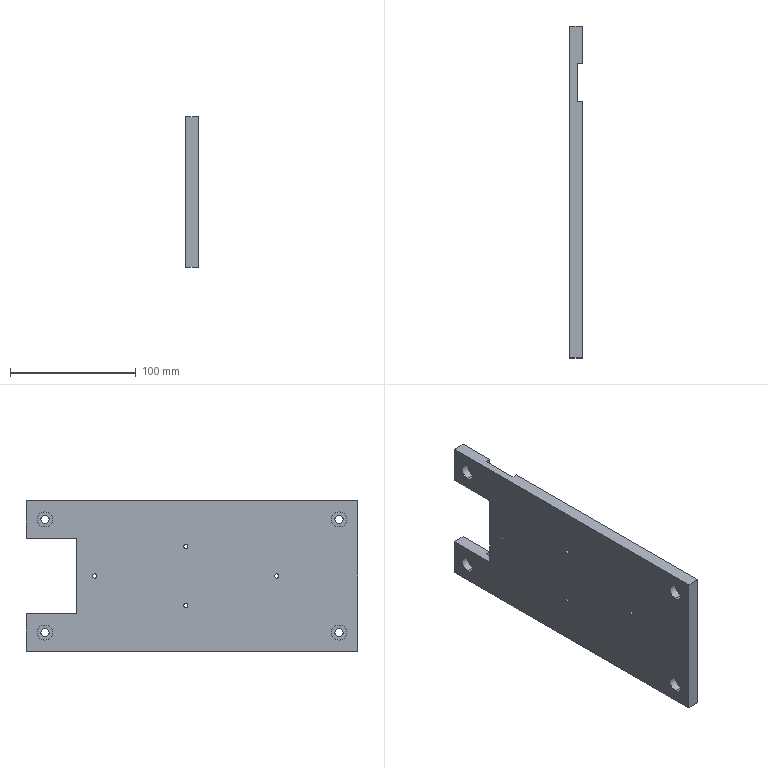Part | STEP file | 02-17 Pusher cylinder fixing plate | 1 solid | 44 faces | box 10 x 264 x 120 mm | volume 277247 mm3 | cylinder 24 | plane 20 | commonest cylinder face diameters 3.3 x8 6.5 x8 12 x8